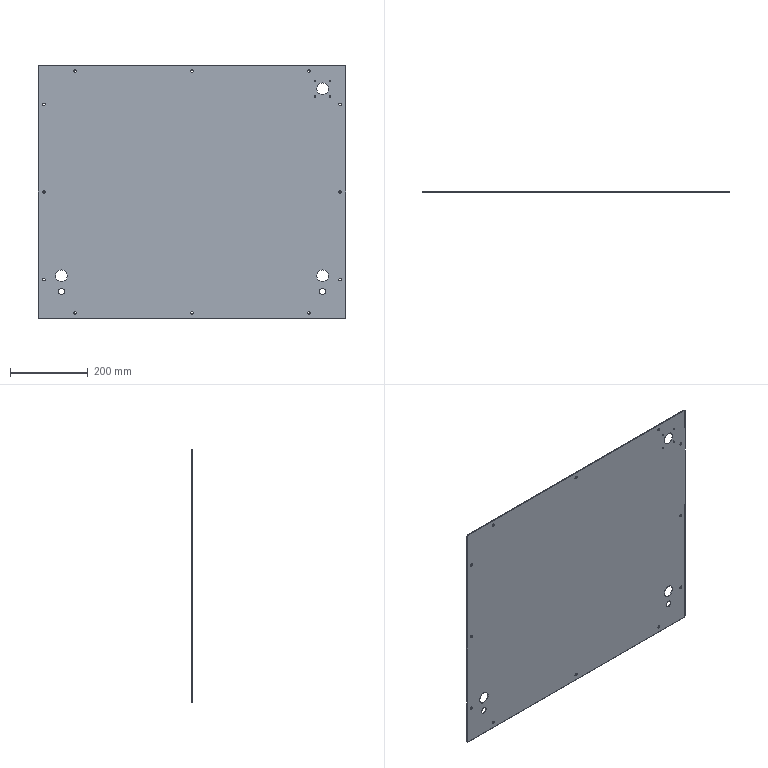Part | STEP file | Top cover plate | 1 solid | 52 faces | box 790 x 1.5 x 650 mm | volume 765787 mm3 | cylinder 46 | plane 6 | commonest cylinder face diameters 6.6 x24 3.3 x8 30 x6 6 x4 16 x4